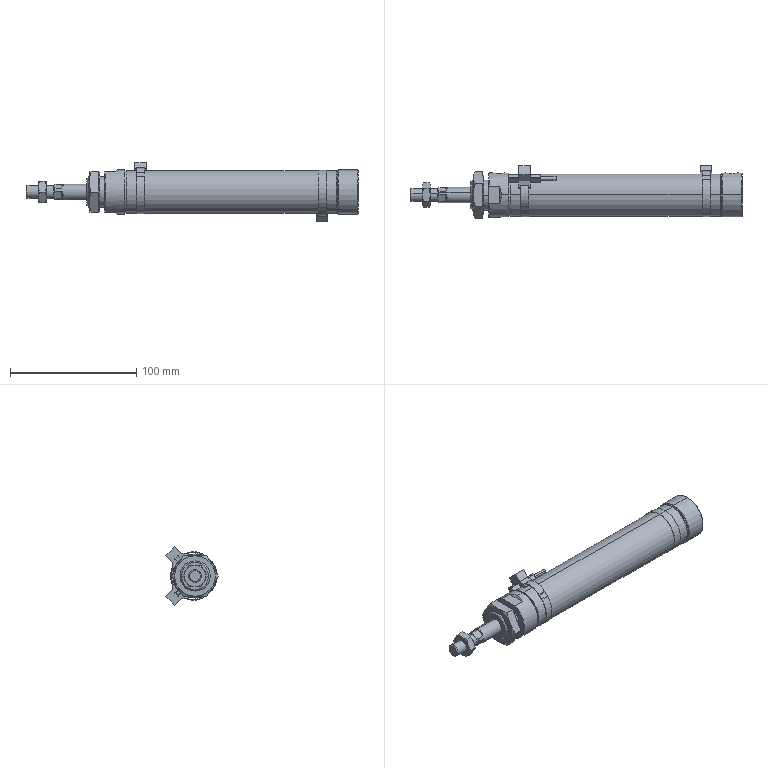Part | SolidWorks | features AEMSimFeature 1 | 6 solids | 224 faces | box 263.352 x 41.739 x 46.528 mm | volume 110258 mm3 | plane 113 | cylinder 60 | cone 43 | torus 8 | commonest cylinder face diameters 28.4 x8 33.6 x6 34.4 x6 1 x4 3 x4 8.566 x4